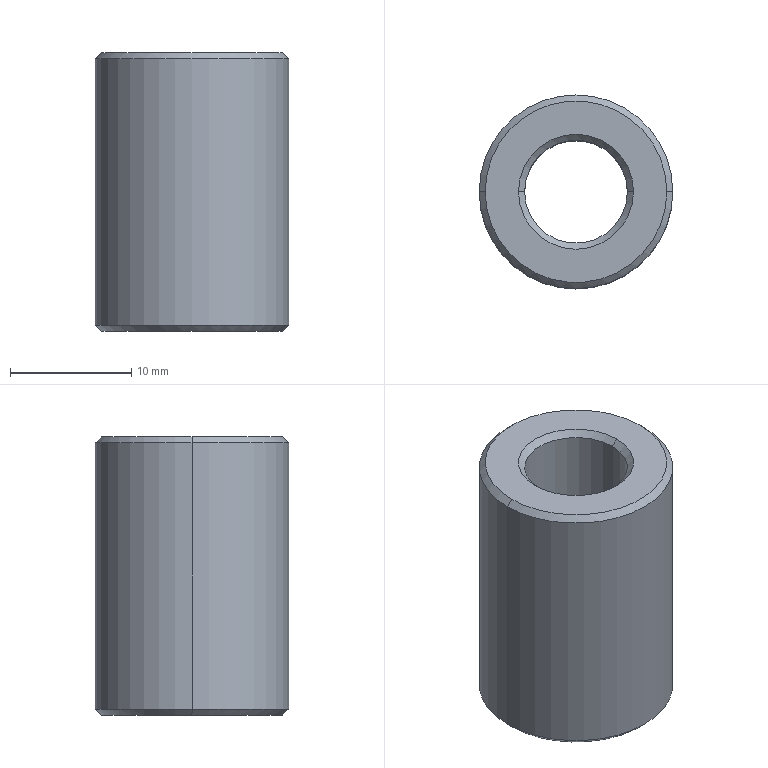Part | STEP file | BPSP-11-19 Cylinder Extension Shaft_Default | 1 solid | 14 faces | box 16 x 16 x 23 mm | volume 3300 mm3 | cone 8 | cylinder 4 | plane 2 | commonest cylinder face diameters 8.5 x2 16 x2
STEP:
#1=CARTESIAN_POINT('',(0.,0.,0.));
#2=DIRECTION('',(0.,0.,1.));
#3=DIRECTION('',(1.,0.,0.));
#4=AXIS2_PLACEMENT_3D('',#1,#2,#3);
#5=CARTESIAN_POINT('',(7.5,0.,23.));
#6=VERTEX_POINT('',#5);
#7=CARTESIAN_POINT('',(-7.5,0.,23.));
#8=VERTEX_POINT('',#7);
#9=CARTESIAN_POINT('',(0.,0.,23.));
#10=DIRECTION('',(0.,0.,1.));
#11=DIRECTION('',(1.,0.,0.));
#12=AXIS2_PLACEMENT_3D('',#9,#10,#11);
#13=CIRCLE('',#12,7.5);
#14=CARTESIAN_POINT('',(0.,0.,23.));
#15=DIRECTION('',(0.,0.,-1.));
#16=DIRECTION('',(-1.,0.,0.));
#17=AXIS2_PLACEMENT_3D('',#14,#15,#16);
#18=CONICAL_SURFACE('',#17,7.5,0.7854);
#19=CARTESIAN_POINT('',(3.142,0.));
#20=DIRECTION('',(-1.,0.));
#21=VECTOR('',#20,1.);
#22=LINE('',#19,#21);
#23=(GEOMETRIC_REPRESENTATION_CONTEXT(2)PARAMETRIC_REPRESENTATION_CONTEXT()REPRESENTATION_CONTEXT('',''));
#24=DEFINITIONAL_REPRESENTATION('',(#22),#23);
#25=PCURVE('',#18,#24);
#26=CARTESIAN_POINT('',(0.,0.,23.));
#27=DIRECTION('',(0.,0.,1.));
#28=DIRECTION('',(1.,0.,0.));
#29=AXIS2_PLACEMENT_3D('',#26,#27,#28);
#30=PLANE('',#29);
#31=CARTESIAN_POINT('',(0.,0.));
#32=DIRECTION('',(1.,0.));
#33=AXIS2_PLACEMENT_2D('',#31,#32);
#34=CIRCLE('',#33,7.5);
#35=(GEOMETRIC_REPRESENTATION_CONTEXT(2)PARAMETRIC_REPRESENTATION_CONTEXT()REPRESENTATION_CONTEXT('',''));
#36=DEFINITIONAL_REPRESENTATION('',(#34),#35);
#37=PCURVE('',#30,#36);
#38=SURFACE_CURVE('',#13,(#25,#37),.PCURVE_S1.);
#39=EDGE_CURVE('',#6,#8,#38,.T.);
#40=ORIENTED_EDGE('',*,*,#39,.F.);
#41=CARTESIAN_POINT('',(8.,0.,22.5));
#42=VERTEX_POINT('',#41);
#43=CARTESIAN_POINT('',(7.5,0.,23.));
#44=DIRECTION('',(0.7071,0.,-0.7071));
#45=VECTOR('',#44,1.);
#46=LINE('',#43,#45);
#47=CARTESIAN_POINT('',(3.142,0.));
#48=DIRECTION('',(0.,1.));
#49=VECTOR('',#48,1.);
#50=LINE('',#47,#49);
#51=(GEOMETRIC_REPRESENTATION_CONTEXT(2)PARAMETRIC_REPRESENTATION_CONTEXT()REPRESENTATION_CONTEXT('',''));
#52=DEFINITIONAL_REPRESENTATION('',(#50),#51);
#53=PCURVE('',#18,#52);
#54=CARTESIAN_POINT('',(0.,0.,23.));
#55=DIRECTION('',(0.,0.,-1.));
#56=DIRECTION('',(-1.,0.,0.));
#57=AXIS2_PLACEMENT_3D('',#54,#55,#56);
#58=CONICAL_SURFACE('',#57,7.5,0.7854);
#59=CARTESIAN_POINT('',(3.142,0.));
#60=DIRECTION('',(0.,1.));
#61=VECTOR('',#60,1.);
#62=LINE('',#59,#61);
#63=(GEOMETRIC_REPRESENTATION_CONTEXT(2)PARAMETRIC_REPRESENTATION_CONTEXT()REPRESENTATION_CONTEXT('',''));
#64=DEFINITIONAL_REPRESENTATION('',(#62),#63);
#65=PCURVE('',#58,#64);
#66=SURFACE_CURVE('',#46,(#53,#65),.PCURVE_S1.);
#67=EDGE_CURVE('',#6,#42,#66,.T.);
#68=ORIENTED_EDGE('',*,*,#67,.T.);
#69=CARTESIAN_POINT('',(-8.,0.,22.5));
#70=VERTEX_POINT('',#69);
#71=CARTESIAN_POINT('',(0.,0.,22.5));
#72=DIRECTION('',(0.,0.,-1.));
#73=DIRECTION('',(1.,0.,0.));
#74=AXIS2_PLACEMENT_3D('',#71,#72,#73);
#75=CIRCLE('',#74,8.);
#76=CARTESIAN_POINT('',(-3.142,0.5));
#77=DIRECTION('',(1.,0.));
#78=VECTOR('',#77,1.);
#79=LINE('',#76,#78);
#80=(GEOMETRIC_REPRESENTATION_CONTEXT(2)PARAMETRIC_REPRESENTATION_CONTEXT()REPRESENTATION_CONTEXT('',''));
#81=DEFINITIONAL_REPRESENTATION('',(#79),#80);
#82=PCURVE('',#18,#81);
#83=CARTESIAN_POINT('',(0.,0.,23.));
#84=DIRECTION('',(0.,0.,-1.));
#85=DIRECTION('',(-1.,0.,0.));
#86=AXIS2_PLACEMENT_3D('',#83,#84,#85);
#87=CYLINDRICAL_SURFACE('',#86,8.);
#88=CARTESIAN_POINT('',(-3.142,0.5));
#89=DIRECTION('',(1.,0.));
#90=VECTOR('',#89,1.);
#91=LINE('',#88,#90);
#92=(GEOMETRIC_REPRESENTATION_CONTEXT(2)PARAMETRIC_REPRESENTATION_CONTEXT()REPRESENTATION_CONTEXT('',''));
#93=DEFINITIONAL_REPRESENTATION('',(#91),#92);
#94=PCURVE('',#87,#93);
#95=SURFACE_CURVE('',#75,(#82,#94),.PCURVE_S1.);
#96=EDGE_CURVE('',#70,#42,#95,.T.);
#97=ORIENTED_EDGE('',*,*,#96,.F.);
#98=CARTESIAN_POINT('',(-7.5,0.,23.));
#99=DIRECTION('',(-0.7071,0.,-0.7071));
#100=VECTOR('',#99,1.);
#101=LINE('',#98,#100);
#102=CARTESIAN_POINT('',(0.,0.));
#103=DIRECTION('',(0.,1.));
#104=VECTOR('',#103,1.);
#105=LINE('',#102,#104);
#106=(GEOMETRIC_REPRESENTATION_CONTEXT(2)PARAMETRIC_REPRESENTATION_CONTEXT()REPRESENTATION_CONTEXT('',''));
#107=DEFINITIONAL_REPRESENTATION('',(#105),#106);
#108=PCURVE('',#18,#107);
#109=CARTESIAN_POINT('',(6.283,0.));
#110=DIRECTION('',(0.,1.));
#111=VECTOR('',#110,1.);
#112=LINE('',#109,#111);
#113=(GEOMETRIC_REPRESENTATION_CONTEXT(2)PARAMETRIC_REPRESENTATION_CONTEXT()REPRESENTATION_CONTEXT('',''));
#114=DEFINITIONAL_REPRESENTATION('',(#112),#113);
#115=PCURVE('',#58,#114);
#116=SURFACE_CURVE('',#101,(#108,#115),.PCURVE_S1.);
#117=EDGE_CURVE('',#8,#70,#116,.T.);
#118=ORIENTED_EDGE('',*,*,#117,.F.);
#119=EDGE_LOOP('',(#40,#68,#97,#118));
#120=FACE_BOUND('',#119,.T.);
#121=ADVANCED_FACE('',(#120),#18,.T.);
#122=CARTESIAN_POINT('',(-7.5,0.,0.));
#123=VERTEX_POINT('',#122);
#124=CARTESIAN_POINT('',(7.5,0.,0.));
#125=VERTEX_POINT('',#124);
#126=CARTESIAN_POINT('',(0.,0.,0.));
#127=DIRECTION('',(0.,0.,-1.));
#128=DIRECTION('',(1.,0.,0.));
#129=AXIS2_PLACEMENT_3D('',#126,#127,#128);
#130=CIRCLE('',#129,7.5);
#131=CARTESIAN_POINT('',(0.,0.,0.5));
#132=DIRECTION('',(0.,0.,1.));
#133=DIRECTION('',(1.,0.,0.));
#134=AXIS2_PLACEMENT_3D('',#131,#132,#133);
#135=CONICAL_SURFACE('',#134,8.,0.7854);
#136=CARTESIAN_POINT('',(6.283,-0.5));
#137=DIRECTION('',(-1.,0.));
#138=VECTOR('',#137,1.);
#139=LINE('',#136,#138);
#140=(GEOMETRIC_REPRESENTATION_CONTEXT(2)PARAMETRIC_REPRESENTATION_CONTEXT()REPRESENTATION_CONTEXT('',''));
#141=DEFINITIONAL_REPRESENTATION('',(#139),#140);
#142=PCURVE('',#135,#141);
#143=CARTESIAN_POINT('',(0.,0.,0.));
#144=DIRECTION('',(0.,0.,1.));
#145=DIRECTION('',(1.,0.,0.));
#146=AXIS2_PLACEMENT_3D('',#143,#144,#145);
#147=PLANE('',#146);
#148=CARTESIAN_POINT('',(7.5,0.));
#149=CARTESIAN_POINT('',(7.5,-12.99));
#150=CARTESIAN_POINT('',(-3.75,-6.495));
#151=CARTESIAN_POINT('',(-15.,0.));
#152=CARTESIAN_POINT('',(-3.75,6.495));
#153=CARTESIAN_POINT('',(7.5,12.99));
#154=CARTESIAN_POINT('',(7.5,0.));
#155=(BOUNDED_CURVE()B_SPLINE_CURVE(2,(#148,#149,#150,#151,#152,#153,#154),.UNSPECIFIED.,.T.,.F.)B_SPLINE_CURVE_WITH_KNOTS((1,2,2,2,2,1),(-2.094,0.,2.094,4.189,6.283,8.378),.UNSPECIFIED.)CURVE()GEOMETRIC_REPRESENTATION_ITEM()RATIONAL_B_SPLINE_CURVE((1.,0.5,1.,0.5,1.,0.5,1.))REPRESENTATION_ITEM(''));
#156=(GEOMETRIC_REPRESENTATION_CONTEXT(2)PARAMETRIC_REPRESENTATION_CONTEXT()REPRESENTATION_CONTEXT('',''));
#157=DEFINITIONAL_REPRESENTATION('',(#155),#156);
#158=PCURVE('',#147,#157);
#159=SURFACE_CURVE('',#130,(#142,#158),.PCURVE_S1.);
#160=EDGE_CURVE('',#123,#125,#159,.T.);
#161=ORIENTED_EDGE('',*,*,#160,.F.);
#162=CARTESIAN_POINT('',(-8.,0.,0.5));
#163=VERTEX_POINT('',#162);
#164=CARTESIAN_POINT('',(-8.,0.,0.5));
#165=DIRECTION('',(-0.7071,0.,0.7071));
#166=VECTOR('',#165,1.);
#167=LINE('',#164,#166);
#168=CARTESIAN_POINT('',(3.142,0.));
#169=DIRECTION('',(0.,1.));
#170=VECTOR('',#169,1.);
#171=LINE('',#168,#170);
#172=(GEOMETRIC_REPRESENTATION_CONTEXT(2)PARAMETRIC_REPRESENTATION_CONTEXT()REPRESENTATION_CONTEXT('',''));
#173=DEFINITIONAL_REPRESENTATION('',(#171),#172);
#174=PCURVE('',#135,#173);
#175=CARTESIAN_POINT('',(0.,0.,0.5));
#176=DIRECTION('',(0.,0.,1.));
#177=DIRECTION('',(1.,0.,0.));
#178=AXIS2_PLACEMENT_3D('',#175,#176,#177);
#179=CONICAL_SURFACE('',#178,8.,0.7854);
#180=CARTESIAN_POINT('',(3.142,0.));
#181=DIRECTION('',(0.,1.));
#182=VECTOR('',#181,1.);
#183=LINE('',#180,#182);
#184=(GEOMETRIC_REPRESENTATION_CONTEXT(2)PARAMETRIC_REPRESENTATION_CONTEXT()REPRESENTATION_CONTEXT('',''));
#185=DEFINITIONAL_REPRESENTATION('',(#183),#184);
#186=PCURVE('',#179,#185);
#187=SURFACE_CURVE('',#167,(#174,#186),.PCURVE_S1.);
#188=EDGE_CURVE('',#123,#163,#187,.T.);
#189=ORIENTED_EDGE('',*,*,#188,.T.);
#190=CARTESIAN_POINT('',(8.,0.,0.5));
#191=VERTEX_POINT('',#190);
#192=CARTESIAN_POINT('',(0.,0.,0.5));
#193=DIRECTION('',(0.,0.,1.));
#194=DIRECTION('',(1.,0.,0.));
#195=AXIS2_PLACEMENT_3D('',#192,#193,#194);
#196=CIRCLE('',#195,8.);
#197=CARTESIAN_POINT('',(0.,0.));
#198=DIRECTION('',(1.,0.));
#199=VECTOR('',#198,1.);
#200=LINE('',#197,#199);
#201=(GEOMETRIC_REPRESENTATION_CONTEXT(2)PARAMETRIC_REPRESENTATION_CONTEXT()REPRESENTATION_CONTEXT('',''));
#202=DEFINITIONAL_REPRESENTATION('',(#200),#201);
#203=PCURVE('',#135,#202);
#204=CARTESIAN_POINT('',(3.142,22.5));
#205=DIRECTION('',(-1.,0.));
#206=VECTOR('',#205,1.);
#207=LINE('',#204,#206);
#208=(GEOMETRIC_REPRESENTATION_CONTEXT(2)PARAMETRIC_REPRESENTATION_CONTEXT()REPRESENTATION_CONTEXT('',''));
#209=DEFINITIONAL_REPRESENTATION('',(#207),#208);
#210=PCURVE('',#87,#209);
#211=SURFACE_CURVE('',#196,(#203,#210),.PCURVE_S1.);
#212=EDGE_CURVE('',#191,#163,#211,.T.);
#213=ORIENTED_EDGE('',*,*,#212,.F.);
#214=CARTESIAN_POINT('',(8.,0.,0.5));
#215=DIRECTION('',(0.7071,0.,0.7071));
#216=VECTOR('',#215,1.);
#217=LINE('',#214,#216);
#218=CARTESIAN_POINT('',(0.,0.));
#219=DIRECTION('',(0.,1.));
#220=VECTOR('',#219,1.);
#221=LINE('',#218,#220);
#222=(GEOMETRIC_REPRESENTATION_CONTEXT(2)PARAMETRIC_REPRESENTATION_CONTEXT()REPRESENTATION_CONTEXT('',''));
#223=DEFINITIONAL_REPRESENTATION('',(#221),#222);
#224=PCURVE('',#135,#223);
#225=CARTESIAN_POINT('',(6.283,0.));
#226=DIRECTION('',(0.,1.));
#227=VECTOR('',#226,1.);
#228=LINE('',#225,#227);
#229=(GEOMETRIC_REPRESENTATION_CONTEXT(2)PARAMETRIC_REPRESENTATION_CONTEXT()REPRESENTATION_CONTEXT('',''));
#230=DEFINITIONAL_REPRESENTATION('',(#228),#229);
#231=PCURVE('',#179,#230);
#232=SURFACE_CURVE('',#217,(#224,#231),.PCURVE_S1.);
#233=EDGE_CURVE('',#125,#191,#232,.T.);
#234=ORIENTED_EDGE('',*,*,#233,.F.);
#235=EDGE_LOOP('',(#161,#189,#213,#234));
#236=FACE_BOUND('',#235,.T.);
#237=ADVANCED_FACE('',(#236),#135,.T.);
#238=CARTESIAN_POINT('',(4.25,0.,22.5));
#239=VERTEX_POINT('',#238);
#240=CARTESIAN_POINT('',(4.75,0.,23.));
#241=VERTEX_POINT('',#240);
#242=CARTESIAN_POINT('',(4.25,0.,22.5));
#243=DIRECTION('',(0.7071,0.,0.7071));
#244=VECTOR('',#243,1.);
#245=LINE('',#242,#244);
#246=CARTESIAN_POINT('',(0.,0.,22.5));
#247=DIRECTION('',(0.,0.,1.));
#248=DIRECTION('',(1.,0.,0.));
#249=AXIS2_PLACEMENT_3D('',#246,#247,#248);
#250=CONICAL_SURFACE('',#249,4.25,0.7854);
#251=CARTESIAN_POINT('',(6.283,0.));
#252=DIRECTION('',(0.,1.));
#253=VECTOR('',#252,1.);
#254=LINE('',#251,#253);
#255=(GEOMETRIC_REPRESENTATION_CONTEXT(2)PARAMETRIC_REPRESENTATION_CONTEXT()REPRESENTATION_CONTEXT('',''));
#256=DEFINITIONAL_REPRESENTATION('',(#254),#255);
#257=PCURVE('',#250,#256);
#258=CARTESIAN_POINT('',(0.,0.,22.5));
#259=DIRECTION('',(0.,0.,1.));
#260=DIRECTION('',(1.,0.,0.));
#261=AXIS2_PLACEMENT_3D('',#258,#259,#260);
#262=CONICAL_SURFACE('',#261,4.25,0.7854);
#263=CARTESIAN_POINT('',(0.,0.));
#264=DIRECTION('',(0.,1.));
#265=VECTOR('',#264,1.);
#266=LINE('',#263,#265);
#267=(GEOMETRIC_REPRESENTATION_CONTEXT(2)PARAMETRIC_REPRESENTATION_CONTEXT()REPRESENTATION_CONTEXT('',''));
#268=DEFINITIONAL_REPRESENTATION('',(#266),#267);
#269=PCURVE('',#262,#268);
#270=SURFACE_CURVE('',#245,(#257,#269),.PCURVE_S1.);
#271=EDGE_CURVE('',#239,#241,#270,.T.);
#272=ORIENTED_EDGE('',*,*,#271,.T.);
#273=CARTESIAN_POINT('',(-4.75,0.,23.));
#274=VERTEX_POINT('',#273);
#275=CARTESIAN_POINT('',(0.,0.,23.));
#276=DIRECTION('',(0.,0.,-1.));
#277=DIRECTION('',(1.,0.,0.));
#278=AXIS2_PLACEMENT_3D('',#275,#276,#277);
#279=CIRCLE('',#278,4.75);
#280=CARTESIAN_POINT('',(6.283,0.5));
#281=DIRECTION('',(-1.,0.));
#282=VECTOR('',#281,1.);
#283=LINE('',#280,#282);
#284=(GEOMETRIC_REPRESENTATION_CONTEXT(2)PARAMETRIC_REPRESENTATION_CONTEXT()REPRESENTATION_CONTEXT('',''));
#285=DEFINITIONAL_REPRESENTATION('',(#283),#284);
#286=PCURVE('',#250,#285);
#287=CARTESIAN_POINT('',(4.75,0.));
#288=CARTESIAN_POINT('',(4.75,-8.227));
#289=CARTESIAN_POINT('',(-2.375,-4.114));
#290=CARTESIAN_POINT('',(-9.5,0.));
#291=CARTESIAN_POINT('',(-2.375,4.114));
#292=CARTESIAN_POINT('',(4.75,8.227));
#293=CARTESIAN_POINT('',(4.75,0.));
#294=(BOUNDED_CURVE()B_SPLINE_CURVE(2,(#287,#288,#289,#290,#291,#292,#293),.UNSPECIFIED.,.T.,.F.)B_SPLINE_CURVE_WITH_KNOTS((1,2,2,2,2,1),(-2.094,0.,2.094,4.189,6.283,8.378),.UNSPECIFIED.)CURVE()GEOMETRIC_REPRESENTATION_ITEM()RATIONAL_B_SPLINE_CURVE((1.,0.5,1.,0.5,1.,0.5,1.))REPRESENTATION_ITEM(''));
#295=(GEOMETRIC_REPRESENTATION_CONTEXT(2)PARAMETRIC_REPRESENTATION_CONTEXT()REPRESENTATION_CONTEXT('',''));
#296=DEFINITIONAL_REPRESENTATION('',(#294),#295);
#297=PCURVE('',#30,#296);
#298=SURFACE_CURVE('',#279,(#286,#297),.PCURVE_S1.);
#299=EDGE_CURVE('',#241,#274,#298,.T.);
#300=ORIENTED_EDGE('',*,*,#299,.T.);
#301=CARTESIAN_POINT('',(-4.25,0.,22.5));
#302=VERTEX_POINT('',#301);
#303=CARTESIAN_POINT('',(-4.25,0.,22.5));
#304=DIRECTION('',(-0.7071,0.,0.7071));
#305=VECTOR('',#304,1.);
#306=LINE('',#303,#305);
#307=CARTESIAN_POINT('',(3.142,0.));
#308=DIRECTION('',(0.,1.));
#309=VECTOR('',#308,1.);
#310=LINE('',#307,#309);
#311=(GEOMETRIC_REPRESENTATION_CONTEXT(2)PARAMETRIC_REPRESENTATION_CONTEXT()REPRESENTATION_CONTEXT('',''));
#312=DEFINITIONAL_REPRESENTATION('',(#310),#311);
#313=PCURVE('',#250,#312);
#314=CARTESIAN_POINT('',(3.142,0.));
#315=DIRECTION('',(0.,1.));
#316=VECTOR('',#315,1.);
#317=LINE('',#314,#316);
#318=(GEOMETRIC_REPRESENTATION_CONTEXT(2)PARAMETRIC_REPRESENTATION_CONTEXT()REPRESENTATION_CONTEXT('',''));
#319=DEFINITIONAL_REPRESENTATION('',(#317),#318);
#320=PCURVE('',#262,#319);
#321=SURFACE_CURVE('',#306,(#313,#320),.PCURVE_S1.);
#322=EDGE_CURVE('',#302,#274,#321,.T.);
#323=ORIENTED_EDGE('',*,*,#322,.F.);
#324=CARTESIAN_POINT('',(0.,0.,22.5));
#325=DIRECTION('',(0.,0.,1.));
#326=DIRECTION('',(1.,0.,0.));
#327=AXIS2_PLACEMENT_3D('',#324,#325,#326);
#328=CIRCLE('',#327,4.25);
#329=CARTESIAN_POINT('',(0.,0.));
#330=DIRECTION('',(1.,0.));
#331=VECTOR('',#330,1.);
#332=LINE('',#329,#331);
#333=(GEOMETRIC_REPRESENTATION_CONTEXT(2)PARAMETRIC_REPRESENTATION_CONTEXT()REPRESENTATION_CONTEXT('',''));
#334=DEFINITIONAL_REPRESENTATION('',(#332),#333);
#335=PCURVE('',#250,#334);
#336=CARTESIAN_POINT('',(0.,0.,23.));
#337=DIRECTION('',(0.,0.,-1.));
#338=DIRECTION('',(-1.,0.,0.));
#339=AXIS2_PLACEMENT_3D('',#336,#337,#338);
#340=CYLINDRICAL_SURFACE('',#339,4.25);
#341=CARTESIAN_POINT('',(9.425,0.5));
#342=DIRECTION('',(-1.,0.));
#343=VECTOR('',#342,1.);
#344=LINE('',#341,#343);
#345=(GEOMETRIC_REPRESENTATION_CONTEXT(2)PARAMETRIC_REPRESENTATION_CONTEXT()REPRESENTATION_CONTEXT('',''));
#346=DEFINITIONAL_REPRESENTATION('',(#344),#345);
#347=PCURVE('',#340,#346);
#348=SURFACE_CURVE('',#328,(#335,#347),.PCURVE_S1.);
#349=EDGE_CURVE('',#302,#239,#348,.T.);
#350=ORIENTED_EDGE('',*,*,#349,.T.);
#351=EDGE_LOOP('',(#272,#300,#323,#350));
#352=FACE_BOUND('',#351,.F.);
#353=ADVANCED_FACE('',(#352),#250,.F.);
#354=CARTESIAN_POINT('',(-4.25,0.,0.5));
#355=VERTEX_POINT('',#354);
#356=CARTESIAN_POINT('',(-4.75,0.,0.));
#357=VERTEX_POINT('',#356);
#358=CARTESIAN_POINT('',(-4.75,0.,0.));
#359=DIRECTION('',(-0.7071,0.,-0.7071));
#360=VECTOR('',#359,1.);
#361=LINE('',#358,#360);
#362=CARTESIAN_POINT('',(0.,0.,0.));
#363=DIRECTION('',(0.,0.,-1.));
#364=DIRECTION('',(-1.,0.,0.));
#365=AXIS2_PLACEMENT_3D('',#362,#363,#364);
#366=CONICAL_SURFACE('',#365,4.75,0.7854);
#367=CARTESIAN_POINT('',(6.283,0.));
#368=DIRECTION('',(0.,1.));
#369=VECTOR('',#368,1.);
#370=LINE('',#367,#369);
#371=(GEOMETRIC_REPRESENTATION_CONTEXT(2)PARAMETRIC_REPRESENTATION_CONTEXT()REPRESENTATION_CONTEXT('',''));
#372=DEFINITIONAL_REPRESENTATION('',(#370),#371);
#373=PCURVE('',#366,#372);
#374=CARTESIAN_POINT('',(0.,0.,0.));
#375=DIRECTION('',(0.,0.,-1.));
#376=DIRECTION('',(-1.,0.,0.));
#377=AXIS2_PLACEMENT_3D('',#374,#375,#376);
#378=CONICAL_SURFACE('',#377,4.75,0.7854);
#379=CARTESIAN_POINT('',(0.,0.));
#380=DIRECTION('',(0.,1.));
#381=VECTOR('',#380,1.);
#382=LINE('',#379,#381);
#383=(GEOMETRIC_REPRESENTATION_CONTEXT(2)PARAMETRIC_REPRESENTATION_CONTEXT()REPRESENTATION_CONTEXT('',''));
#384=DEFINITIONAL_REPRESENTATION('',(#382),#383);
#385=PCURVE('',#378,#384);
#386=SURFACE_CURVE('',#361,(#373,#385),.PCURVE_S1.);
#387=EDGE_CURVE('',#355,#357,#386,.T.);
#388=ORIENTED_EDGE('',*,*,#387,.T.);
#389=CARTESIAN_POINT('',(4.75,0.,0.));
#390=VERTEX_POINT('',#389);
#391=CARTESIAN_POINT('',(0.,0.,0.));
#392=DIRECTION('',(0.,0.,1.));
#393=DIRECTION('',(1.,0.,0.));
#394=AXIS2_PLACEMENT_3D('',#391,#392,#393);
#395=CIRCLE('',#394,4.75);
#396=CARTESIAN_POINT('',(9.425,0.));
#397=DIRECTION('',(-1.,0.));
#398=VECTOR('',#397,1.);
#399=LINE('',#396,#398);
#400=(GEOMETRIC_REPRESENTATION_CONTEXT(2)PARAMETRIC_REPRESENTATION_CONTEXT()REPRESENTATION_CONTEXT('',''));
#401=DEFINITIONAL_REPRESENTATION('',(#399),#400);
#402=PCURVE('',#366,#401);
#403=CARTESIAN_POINT('',(0.,0.));
#404=DIRECTION('',(1.,0.));
#405=AXIS2_PLACEMENT_2D('',#403,#404);
#406=CIRCLE('',#405,4.75);
#407=(GEOMETRIC_REPRESENTATION_CONTEXT(2)PARAMETRIC_REPRESENTATION_CONTEXT()REPRESENTATION_CONTEXT('',''));
#408=DEFINITIONAL_REPRESENTATION('',(#406),#407);
#409=PCURVE('',#147,#408);
#410=SURFACE_CURVE('',#395,(#402,#409),.PCURVE_S1.);
#411=EDGE_CURVE('',#357,#390,#410,.T.);
#412=ORIENTED_EDGE('',*,*,#411,.T.);
#413=CARTESIAN_POINT('',(4.25,0.,0.5));
#414=VERTEX_POINT('',#413);
#415=CARTESIAN_POINT('',(4.75,0.,0.));
#416=DIRECTION('',(0.7071,0.,-0.7071));
#417=VECTOR('',#416,1.);
#418=LINE('',#415,#417);
#419=CARTESIAN_POINT('',(3.142,0.));
#420=DIRECTION('',(0.,1.));
#421=VECTOR('',#420,1.);
#422=LINE('',#419,#421);
#423=(GEOMETRIC_REPRESENTATION_CONTEXT(2)PARAMETRIC_REPRESENTATION_CONTEXT()REPRESENTATION_CONTEXT('',''));
#424=DEFINITIONAL_REPRESENTATION('',(#422),#423);
#425=PCURVE('',#366,#424);
#426=CARTESIAN_POINT('',(3.142,0.));
#427=DIRECTION('',(0.,1.));
#428=VECTOR('',#427,1.);
#429=LINE('',#426,#428);
#430=(GEOMETRIC_REPRESENTATION_CONTEXT(2)PARAMETRIC_REPRESENTATION_CONTEXT()REPRESENTATION_CONTEXT('',''));
#431=DEFINITIONAL_REPRESENTATION('',(#429),#430);
#432=PCURVE('',#378,#431);
#433=SURFACE_CURVE('',#418,(#425,#432),.PCURVE_S1.);
#434=EDGE_CURVE('',#414,#390,#433,.T.);
#435=ORIENTED_EDGE('',*,*,#434,.F.);
#436=CARTESIAN_POINT('',(0.,0.,0.5));
#437=DIRECTION('',(0.,0.,-1.));
#438=DIRECTION('',(1.,0.,0.));
#439=AXIS2_PLACEMENT_3D('',#436,#437,#438);
#440=CIRCLE('',#439,4.25);
#441=CARTESIAN_POINT('',(3.142,-0.5));
#442=DIRECTION('',(1.,0.));
#443=VECTOR('',#442,1.);
#444=LINE('',#441,#443);
#445=(GEOMETRIC_REPRESENTATION_CONTEXT(2)PARAMETRIC_REPRESENTATION_CONTEXT()REPRESENTATION_CONTEXT('',''));
#446=DEFINITIONAL_REPRESENTATION('',(#444),#445);
#447=PCURVE('',#366,#446);
#448=CARTESIAN_POINT('',(3.142,22.5));
#449=DIRECTION('',(1.,0.));
#450=VECTOR('',#449,1.);
#451=LINE('',#448,#450);
#452=(GEOMETRIC_REPRESENTATION_CONTEXT(2)PARAMETRIC_REPRESENTATION_CONTEXT()REPRESENTATION_CONTEXT('',''));
#453=DEFINITIONAL_REPRESENTATION('',(#451),#452);
#454=PCURVE('',#340,#453);
#455=SURFACE_CURVE('',#440,(#447,#454),.PCURVE_S1.);
#456=EDGE_CURVE('',#414,#355,#455,.T.);
#457=ORIENTED_EDGE('',*,*,#456,.T.);
#458=EDGE_LOOP('',(#388,#412,#435,#457));
#459=FACE_BOUND('',#458,.F.);
#460=ADVANCED_FACE('',(#459),#366,.F.);
#461=CARTESIAN_POINT('',(-4.25,0.,23.));
#462=DIRECTION('',(0.,0.,-1.));
#463=VECTOR('',#462,1.);
#464=LINE('',#461,#463);
#465=CARTESIAN_POINT('',(6.283,0.));
#466=DIRECTION('',(0.,1.));
#467=VECTOR('',#466,1.);
#468=LINE('',#465,#467);
#469=(GEOMETRIC_REPRESENTATION_CONTEXT(2)PARAMETRIC_REPRESENTATION_CONTEXT()REPRESENTATION_CONTEXT('',''));
#470=DEFINITIONAL_REPRESENTATION('',(#468),#469);
#471=PCURVE('',#340,#470);
#472=CARTESIAN_POINT('',(0.,0.,23.));
#473=DIRECTION('',(0.,0.,-1.));
#474=DIRECTION('',(-1.,0.,0.));
#475=AXIS2_PLACEMENT_3D('',#472,#473,#474);
#476=CYLINDRICAL_SURFACE('',#475,4.25);
#477=CARTESIAN_POINT('',(0.,0.));
#478=DIRECTION('',(0.,1.));
#479=VECTOR('',#478,1.);
#480=LINE('',#477,#479);
#481=(GEOMETRIC_REPRESENTATION_CONTEXT(2)PARAMETRIC_REPRESENTATION_CONTEXT()REPRESENTATION_CONTEXT('',''));
#482=DEFINITIONAL_REPRESENTATION('',(#480),#481);
#483=PCURVE('',#476,#482);
#484=SURFACE_CURVE('',#464,(#471,#483),.PCURVE_S1.);
#485=EDGE_CURVE('',#302,#355,#484,.T.);
#486=ORIENTED_EDGE('',*,*,#485,.T.);
#487=ORIENTED_EDGE('',*,*,#456,.F.);
#488=CARTESIAN_POINT('',(4.25,0.,23.));
#489=DIRECTION('',(0.,0.,-1.));
#490=VECTOR('',#489,1.);
#491=LINE('',#488,#490);
#492=CARTESIAN_POINT('',(3.142,0.));
#493=DIRECTION('',(0.,1.));
#494=VECTOR('',#493,1.);
#495=LINE('',#492,#494);
#496=(GEOMETRIC_REPRESENTATION_CONTEXT(2)PARAMETRIC_REPRESENTATION_CONTEXT()REPRESENTATION_CONTEXT('',''));
#497=DEFINITIONAL_REPRESENTATION('',(#495),#496);
#498=PCURVE('',#340,#497);
#499=CARTESIAN_POINT('',(3.142,0.));
#500=DIRECTION('',(0.,1.));
#501=VECTOR('',#500,1.);
#502=LINE('',#499,#501);
#503=(GEOMETRIC_REPRESENTATION_CONTEXT(2)PARAMETRIC_REPRESENTATION_CONTEXT()REPRESENTATION_CONTEXT('',''));
#504=DEFINITIONAL_REPRESENTATION('',(#502),#503);
#505=PCURVE('',#476,#504);
#506=SURFACE_CURVE('',#491,(#498,#505),.PCURVE_S1.);
#507=EDGE_CURVE('',#239,#414,#506,.T.);
#508=ORIENTED_EDGE('',*,*,#507,.F.);
#509=ORIENTED_EDGE('',*,*,#349,.F.);
#510=EDGE_LOOP('',(#486,#487,#508,#509));
#511=FACE_BOUND('',#510,.F.);
#512=ADVANCED_FACE('',(#511),#340,.F.);
#513=ORIENTED_EDGE('',*,*,#96,.T.);
#514=CARTESIAN_POINT('',(8.,0.,23.));
#515=DIRECTION('',(0.,0.,-1.));
#516=VECTOR('',#515,1.);
#517=LINE('',#514,#516);
#518=CARTESIAN_POINT('',(3.142,0.));
#519=DIRECTION('',(0.,1.));
#520=VECTOR('',#519,1.);
#521=LINE('',#518,#520);
#522=(GEOMETRIC_REPRESENTATION_CONTEXT(2)PARAMETRIC_REPRESENTATION_CONTEXT()REPRESENTATION_CONTEXT('',''));
#523=DEFINITIONAL_REPRESENTATION('',(#521),#522);
#524=PCURVE('',#87,#523);
#525=CARTESIAN_POINT('',(0.,0.,23.));
#526=DIRECTION('',(0.,0.,-1.));
#527=DIRECTION('',(-1.,0.,0.));
#528=AXIS2_PLACEMENT_3D('',#525,#526,#527);
#529=CYLINDRICAL_SURFACE('',#528,8.);
#530=CARTESIAN_POINT('',(3.142,0.));
#531=DIRECTION('',(0.,1.));
#532=VECTOR('',#531,1.);
#533=LINE('',#530,#532);
#534=(GEOMETRIC_REPRESENTATION_CONTEXT(2)PARAMETRIC_REPRESENTATION_CONTEXT()REPRESENTATION_CONTEXT('',''));
#535=DEFINITIONAL_REPRESENTATION('',(#533),#534);
#536=PCURVE('',#529,#535);
#537=SURFACE_CURVE('',#517,(#524,#536),.PCURVE_S1.);
#538=EDGE_CURVE('',#42,#191,#537,.T.);
#539=ORIENTED_EDGE('',*,*,#538,.T.);
#540=ORIENTED_EDGE('',*,*,#212,.T.);
#541=CARTESIAN_POINT('',(-8.,0.,23.));
#542=DIRECTION('',(0.,0.,-1.));
#543=VECTOR('',#542,1.);
#544=LINE('',#541,#543);
#545=CARTESIAN_POINT('',(0.,0.));
#546=DIRECTION('',(0.,1.));
#547=VECTOR('',#546,1.);
#548=LINE('',#545,#547);
#549=(GEOMETRIC_REPRESENTATION_CONTEXT(2)PARAMETRIC_REPRESENTATION_CONTEXT()REPRESENTATION_CONTEXT('',''));
#550=DEFINITIONAL_REPRESENTATION('',(#548),#549);
#551=PCURVE('',#87,#550);
#552=CARTESIAN_POINT('',(6.283,0.));
#553=DIRECTION('',(0.,1.));
#554=VECTOR('',#553,1.);
#555=LINE('',#552,#554);
#556=(GEOMETRIC_REPRESENTATION_CONTEXT(2)PARAMETRIC_REPRESENTATION_CONTEXT()REPRESENTATION_CONTEXT('',''));
#557=DEFINITIONAL_REPRESENTATION('',(#555),#556);
#558=PCURVE('',#529,#557);
#559=SURFACE_CURVE('',#544,(#551,#558),.PCURVE_S1.);
#560=EDGE_CURVE('',#70,#163,#559,.T.);
#561=ORIENTED_EDGE('',*,*,#560,.F.);
#562=EDGE_LOOP('',(#513,#539,#540,#561));
#563=FACE_BOUND('',#562,.T.);
#564=ADVANCED_FACE('',(#563),#87,.T.);
#565=ORIENTED_EDGE('',*,*,#299,.T.);
#566=CARTESIAN_POINT('',(0.,0.,23.));
#567=DIRECTION('',(0.,0.,-1.));
#568=DIRECTION('',(1.,0.,0.));
#569=AXIS2_PLACEMENT_3D('',#566,#567,#568);
#570=CIRCLE('',#569,4.75);
#571=CARTESIAN_POINT('',(4.75,0.));
#572=CARTESIAN_POINT('',(4.75,-8.227));
#573=CARTESIAN_POINT('',(-2.375,-4.114));
#574=CARTESIAN_POINT('',(-9.5,0.));
#575=CARTESIAN_POINT('',(-2.375,4.114));
#576=CARTESIAN_POINT('',(4.75,8.227));
#577=CARTESIAN_POINT('',(4.75,0.));
#578=(BOUNDED_CURVE()B_SPLINE_CURVE(2,(#571,#572,#573,#574,#575,#576,#577),.UNSPECIFIED.,.T.,.F.)B_SPLINE_CURVE_WITH_KNOTS((1,2,2,2,2,1),(-2.094,0.,2.094,4.189,6.283,8.378),.UNSPECIFIED.)CURVE()GEOMETRIC_REPRESENTATION_ITEM()RATIONAL_B_SPLINE_CURVE((1.,0.5,1.,0.5,1.,0.5,1.))REPRESENTATION_ITEM(''));
#579=(GEOMETRIC_REPRESENTATION_CONTEXT(2)PARAMETRIC_REPRESENTATION_CONTEXT()REPRESENTATION_CONTEXT('',''));
#580=DEFINITIONAL_REPRESENTATION('',(#578),#579);
#581=PCURVE('',#30,#580);
#582=CARTESIAN_POINT('',(6.283,0.5));
#583=DIRECTION('',(-1.,0.));
#584=VECTOR('',#583,1.);
#585=LINE('',#582,#584);
#586=(GEOMETRIC_REPRESENTATION_CONTEXT(2)PARAMETRIC_REPRESENTATION_CONTEXT()REPRESENTATION_CONTEXT('',''));
#587=DEFINITIONAL_REPRESENTATION('',(#585),#586);
#588=PCURVE('',#262,#587);
#589=SURFACE_CURVE('',#570,(#581,#588),.PCURVE_S1.);
#590=EDGE_CURVE('',#274,#241,#589,.T.);
#591=ORIENTED_EDGE('',*,*,#590,.T.);
#592=EDGE_LOOP('',(#565,#591));
#593=FACE_BOUND('',#592,.T.);
#594=CARTESIAN_POINT('',(0.,0.,23.));
#595=DIRECTION('',(0.,0.,1.));
#596=DIRECTION('',(1.,0.,0.));
#597=AXIS2_PLACEMENT_3D('',#594,#595,#596);
#598=CIRCLE('',#597,7.5);
#599=CARTESIAN_POINT('',(0.,0.));
#600=DIRECTION('',(1.,0.));
#601=AXIS2_PLACEMENT_2D('',#599,#600);
#602=CIRCLE('',#601,7.5);
#603=(GEOMETRIC_REPRESENTATION_CONTEXT(2)PARAMETRIC_REPRESENTATION_CONTEXT()REPRESENTATION_CONTEXT('',''));
#604=DEFINITIONAL_REPRESENTATION('',(#602),#603);
#605=PCURVE('',#30,#604);
#606=CARTESIAN_POINT('',(9.425,0.));
#607=DIRECTION('',(-1.,0.));
#608=VECTOR('',#607,1.);
#609=LINE('',#606,#608);
#610=(GEOMETRIC_REPRESENTATION_CONTEXT(2)PARAMETRIC_REPRESENTATION_CONTEXT()REPRESENTATION_CONTEXT('',''));
#611=DEFINITIONAL_REPRESENTATION('',(#609),#610);
#612=PCURVE('',#58,#611);
#613=SURFACE_CURVE('',#598,(#605,#612),.PCURVE_S1.);
#614=EDGE_CURVE('',#8,#6,#613,.T.);
#615=ORIENTED_EDGE('',*,*,#614,.T.);
#616=ORIENTED_EDGE('',*,*,#39,.T.);
#617=EDGE_LOOP('',(#615,#616));
#618=FACE_BOUND('',#617,.T.);
#619=ADVANCED_FACE('',(#593,#618),#30,.T.);
#620=ORIENTED_EDGE('',*,*,#411,.T.);
#621=CARTESIAN_POINT('',(0.,0.,0.));
#622=DIRECTION('',(0.,0.,1.));
#623=DIRECTION('',(1.,0.,0.));
#624=AXIS2_PLACEMENT_3D('',#621,#622,#623);
#625=CIRCLE('',#624,4.75);
#626=CARTESIAN_POINT('',(0.,0.));
#627=DIRECTION('',(1.,0.));
#628=AXIS2_PLACEMENT_2D('',#626,#627);
#629=CIRCLE('',#628,4.75);
#630=(GEOMETRIC_REPRESENTATION_CONTEXT(2)PARAMETRIC_REPRESENTATION_CONTEXT()REPRESENTATION_CONTEXT('',''));
#631=DEFINITIONAL_REPRESENTATION('',(#629),#630);
#632=PCURVE('',#147,#631);
#633=CARTESIAN_POINT('',(3.142,0.));
#634=DIRECTION('',(-1.,0.));
#635=VECTOR('',#634,1.);
#636=LINE('',#633,#635);
#637=(GEOMETRIC_REPRESENTATION_CONTEXT(2)PARAMETRIC_REPRESENTATION_CONTEXT()REPRESENTATION_CONTEXT('',''));
#638=DEFINITIONAL_REPRESENTATION('',(#636),#637);
#639=PCURVE('',#378,#638);
#640=SURFACE_CURVE('',#625,(#632,#639),.PCURVE_S1.);
#641=EDGE_CURVE('',#390,#357,#640,.T.);
#642=ORIENTED_EDGE('',*,*,#641,.T.);
#643=EDGE_LOOP('',(#620,#642));
#644=FACE_BOUND('',#643,.T.);
#645=CARTESIAN_POINT('',(0.,0.,0.));
#646=DIRECTION('',(0.,0.,-1.));
#647=DIRECTION('',(1.,0.,0.));
#648=AXIS2_PLACEMENT_3D('',#645,#646,#647);
#649=CIRCLE('',#648,7.5);
#650=CARTESIAN_POINT('',(7.5,0.));
#651=CARTESIAN_POINT('',(7.5,-12.99));
#652=CARTESIAN_POINT('',(-3.75,-6.495));
#653=CARTESIAN_POINT('',(-15.,0.));
#654=CARTESIAN_POINT('',(-3.75,6.495));
#655=CARTESIAN_POINT('',(7.5,12.99));
#656=CARTESIAN_POINT('',(7.5,0.));
#657=(BOUNDED_CURVE()B_SPLINE_CURVE(2,(#650,#651,#652,#653,#654,#655,#656),.UNSPECIFIED.,.T.,.F.)B_SPLINE_CURVE_WITH_KNOTS((1,2,2,2,2,1),(-2.094,0.,2.094,4.189,6.283,8.378),.UNSPECIFIED.)CURVE()GEOMETRIC_REPRESENTATION_ITEM()RATIONAL_B_SPLINE_CURVE((1.,0.5,1.,0.5,1.,0.5,1.))REPRESENTATION_ITEM(''));
#658=(GEOMETRIC_REPRESENTATION_CONTEXT(2)PARAMETRIC_REPRESENTATION_CONTEXT()REPRESENTATION_CONTEXT('',''));
#659=DEFINITIONAL_REPRESENTATION('',(#657),#658);
#660=PCURVE('',#147,#659);
#661=CARTESIAN_POINT('',(6.283,-0.5));
#662=DIRECTION('',(-1.,0.));
#663=VECTOR('',#662,1.);
#664=LINE('',#661,#663);
#665=(GEOMETRIC_REPRESENTATION_CONTEXT(2)PARAMETRIC_REPRESENTATION_CONTEXT()REPRESENTATION_CONTEXT('',''));
#666=DEFINITIONAL_REPRESENTATION('',(#664),#665);
#667=PCURVE('',#179,#666);
#668=SURFACE_CURVE('',#649,(#660,#667),.PCURVE_S1.);
#669=EDGE_CURVE('',#125,#123,#668,.T.);
#670=ORIENTED_EDGE('',*,*,#669,.T.);
#671=ORIENTED_EDGE('',*,*,#160,.T.);
#672=EDGE_LOOP('',(#670,#671));
#673=FACE_BOUND('',#672,.T.);
#674=ADVANCED_FACE('',(#644,#673),#147,.F.);
#675=ORIENTED_EDGE('',*,*,#538,.F.);
#676=CARTESIAN_POINT('',(0.,0.,22.5));
#677=DIRECTION('',(0.,0.,-1.));
#678=DIRECTION('',(1.,0.,0.));
#679=AXIS2_PLACEMENT_3D('',#676,#677,#678);
#680=CIRCLE('',#679,8.);
#681=CARTESIAN_POINT('',(3.142,0.5));
#682=DIRECTION('',(1.,0.));
#683=VECTOR('',#682,1.);
#684=LINE('',#681,#683);
#685=(GEOMETRIC_REPRESENTATION_CONTEXT(2)PARAMETRIC_REPRESENTATION_CONTEXT()REPRESENTATION_CONTEXT('',''));
#686=DEFINITIONAL_REPRESENTATION('',(#684),#685);
#687=PCURVE('',#529,#686);
#688=CARTESIAN_POINT('',(3.142,0.5));
#689=DIRECTION('',(1.,0.));
#690=VECTOR('',#689,1.);
#691=LINE('',#688,#690);
#692=(GEOMETRIC_REPRESENTATION_CONTEXT(2)PARAMETRIC_REPRESENTATION_CONTEXT()REPRESENTATION_CONTEXT('',''));
#693=DEFINITIONAL_REPRESENTATION('',(#691),#692);
#694=PCURVE('',#58,#693);
#695=SURFACE_CURVE('',#680,(#687,#694),.PCURVE_S1.);
#696=EDGE_CURVE('',#42,#70,#695,.T.);
#697=ORIENTED_EDGE('',*,*,#696,.T.);
#698=ORIENTED_EDGE('',*,*,#560,.T.);
#699=CARTESIAN_POINT('',(0.,0.,0.5));
#700=DIRECTION('',(0.,0.,1.));
#701=DIRECTION('',(1.,0.,0.));
#702=AXIS2_PLACEMENT_3D('',#699,#700,#701);
#703=CIRCLE('',#702,8.);
#704=CARTESIAN_POINT('',(9.425,22.5));
#705=DIRECTION('',(-1.,0.));
#706=VECTOR('',#705,1.);
#707=LINE('',#704,#706);
#708=(GEOMETRIC_REPRESENTATION_CONTEXT(2)PARAMETRIC_REPRESENTATION_CONTEXT()REPRESENTATION_CONTEXT('',''));
#709=DEFINITIONAL_REPRESENTATION('',(#707),#708);
#710=PCURVE('',#529,#709);
#711=CARTESIAN_POINT('',(0.,0.));
#712=DIRECTION('',(1.,0.));
#713=VECTOR('',#712,1.);
#714=LINE('',#711,#713);
#715=(GEOMETRIC_REPRESENTATION_CONTEXT(2)PARAMETRIC_REPRESENTATION_CONTEXT()REPRESENTATION_CONTEXT('',''));
#716=DEFINITIONAL_REPRESENTATION('',(#714),#715);
#717=PCURVE('',#179,#716);
#718=SURFACE_CURVE('',#703,(#710,#717),.PCURVE_S1.);
#719=EDGE_CURVE('',#163,#191,#718,.T.);
#720=ORIENTED_EDGE('',*,*,#719,.T.);
#721=EDGE_LOOP('',(#675,#697,#698,#720));
#722=FACE_BOUND('',#721,.T.);
#723=ADVANCED_FACE('',(#722),#529,.T.);
#724=CARTESIAN_POINT('',(0.,0.,0.5));
#725=DIRECTION('',(0.,0.,-1.));
#726=DIRECTION('',(1.,0.,0.));
#727=AXIS2_PLACEMENT_3D('',#724,#725,#726);
#728=CIRCLE('',#727,4.25);
#729=CARTESIAN_POINT('',(-3.142,22.5));
#730=DIRECTION('',(1.,0.));
#731=VECTOR('',#730,1.);
#732=LINE('',#729,#731);
#733=(GEOMETRIC_REPRESENTATION_CONTEXT(2)PARAMETRIC_REPRESENTATION_CONTEXT()REPRESENTATION_CONTEXT('',''));
#734=DEFINITIONAL_REPRESENTATION('',(#732),#733);
#735=PCURVE('',#476,#734);
#736=CARTESIAN_POINT('',(-3.142,-0.5));
#737=DIRECTION('',(1.,0.));
#738=VECTOR('',#737,1.);
#739=LINE('',#736,#738);
#740=(GEOMETRIC_REPRESENTATION_CONTEXT(2)PARAMETRIC_REPRESENTATION_CONTEXT()REPRESENTATION_CONTEXT('',''));
#741=DEFINITIONAL_REPRESENTATION('',(#739),#740);
#742=PCURVE('',#378,#741);
#743=SURFACE_CURVE('',#728,(#735,#742),.PCURVE_S1.);
#744=EDGE_CURVE('',#355,#414,#743,.T.);
#745=ORIENTED_EDGE('',*,*,#744,.F.);
#746=ORIENTED_EDGE('',*,*,#485,.F.);
#747=CARTESIAN_POINT('',(0.,0.,22.5));
#748=DIRECTION('',(0.,0.,1.));
#749=DIRECTION('',(1.,0.,0.));
#750=AXIS2_PLACEMENT_3D('',#747,#748,#749);
#751=CIRCLE('',#750,4.25);
#752=CARTESIAN_POINT('',(3.142,0.5));
#753=DIRECTION('',(-1.,0.));
#754=VECTOR('',#753,1.);
#755=LINE('',#752,#754);
#756=(GEOMETRIC_REPRESENTATION_CONTEXT(2)PARAMETRIC_REPRESENTATION_CONTEXT()REPRESENTATION_CONTEXT('',''));
#757=DEFINITIONAL_REPRESENTATION('',(#755),#756);
#758=PCURVE('',#476,#757);
#759=CARTESIAN_POINT('',(0.,0.));
#760=DIRECTION('',(1.,0.));
#761=VECTOR('',#760,1.);
#762=LINE('',#759,#761);
#763=(GEOMETRIC_REPRESENTATION_CONTEXT(2)PARAMETRIC_REPRESENTATION_CONTEXT()REPRESENTATION_CONTEXT('',''));
#764=DEFINITIONAL_REPRESENTATION('',(#762),#763);
#765=PCURVE('',#262,#764);
#766=SURFACE_CURVE('',#751,(#758,#765),.PCURVE_S1.);
#767=EDGE_CURVE('',#239,#302,#766,.T.);
#768=ORIENTED_EDGE('',*,*,#767,.F.);
#769=ORIENTED_EDGE('',*,*,#507,.T.);
#770=EDGE_LOOP('',(#745,#746,#768,#769));
#771=FACE_BOUND('',#770,.F.);
#772=ADVANCED_FACE('',(#771),#476,.F.);
#773=ORIENTED_EDGE('',*,*,#641,.T.);
#774=ORIENTED_EDGE('',*,*,#387,.F.);
#775=ORIENTED_EDGE('',*,*,#744,.T.);
#776=ORIENTED_EDGE('',*,*,#434,.T.);
#777=EDGE_LOOP('',(#773,#774,#775,#776));
#778=FACE_BOUND('',#777,.F.);
#779=ADVANCED_FACE('',(#778),#378,.F.);
#780=ORIENTED_EDGE('',*,*,#590,.T.);
#781=ORIENTED_EDGE('',*,*,#271,.F.);
#782=ORIENTED_EDGE('',*,*,#767,.T.);
#783=ORIENTED_EDGE('',*,*,#322,.T.);
#784=EDGE_LOOP('',(#780,#781,#782,#783));
#785=FACE_BOUND('',#784,.F.);
#786=ADVANCED_FACE('',(#785),#262,.F.);
#787=ORIENTED_EDGE('',*,*,#188,.F.);
#788=ORIENTED_EDGE('',*,*,#669,.F.);
#789=ORIENTED_EDGE('',*,*,#233,.T.);
#790=ORIENTED_EDGE('',*,*,#719,.F.);
#791=EDGE_LOOP('',(#787,#788,#789,#790));
#792=FACE_BOUND('',#791,.T.);
#793=ADVANCED_FACE('',(#792),#179,.T.);
#794=ORIENTED_EDGE('',*,*,#67,.F.);
#795=ORIENTED_EDGE('',*,*,#614,.F.);
#796=ORIENTED_EDGE('',*,*,#117,.T.);
#797=ORIENTED_EDGE('',*,*,#696,.F.);
#798=EDGE_LOOP('',(#794,#795,#796,#797));
#799=FACE_BOUND('',#798,.T.);
#800=ADVANCED_FACE('',(#799),#58,.T.);
#801=CLOSED_SHELL('',(#121,#237,#353,#460,#512,#564,#619,#674,#723,#772,#779,#786,#793,#800));
#802=MANIFOLD_SOLID_BREP('',#801);
#803=(LENGTH_UNIT()NAMED_UNIT(*)SI_UNIT(.MILLI.,.METRE.));
#804=UNCERTAINTY_MEASURE_WITH_UNIT(LENGTH_MEASURE(0.0000001),#803,'','');
#805=(NAMED_UNIT(*)PLANE_ANGLE_UNIT()SI_UNIT($,.RADIAN.));
#806=(NAMED_UNIT(*)SI_UNIT($,.STERADIAN.)SOLID_ANGLE_UNIT());
#807=(GEOMETRIC_REPRESENTATION_CONTEXT(3)GLOBAL_UNCERTAINTY_ASSIGNED_CONTEXT((#804))GLOBAL_UNIT_ASSIGNED_CONTEXT((#803,#805,#806))REPRESENTATION_CONTEXT('',''));
#808=ADVANCED_BREP_SHAPE_REPRESENTATION('',(#4,#802),#807);